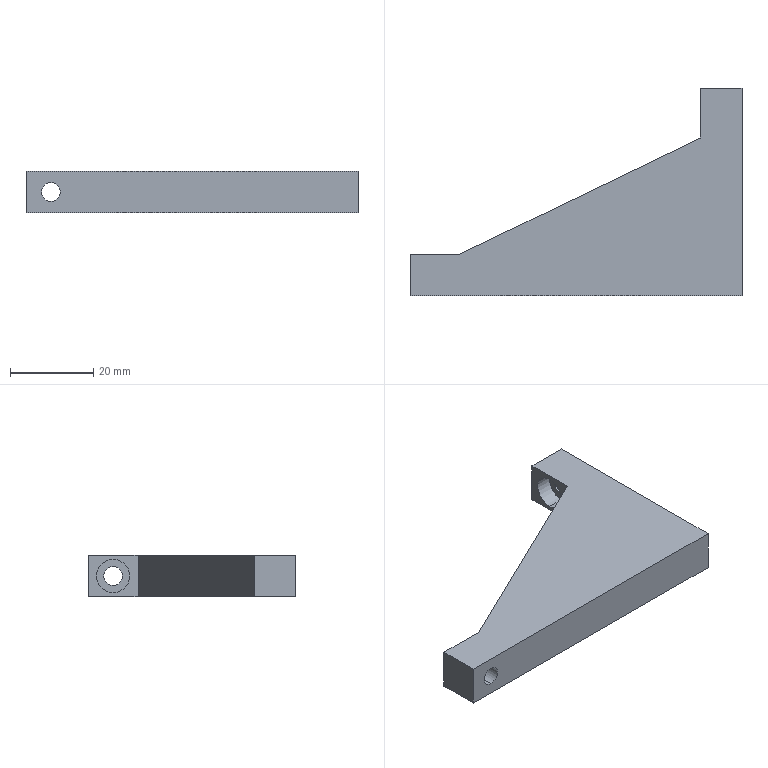Part | NX | features BREP 1 | 1 solid | 19 faces | box 80 x 50 x 10 mm | volume 19527 mm3 | plane 11 | cylinder 8 | commonest cylinder face diameters 4.5 x4 8 x4
STEP:
#1=CARTESIAN_POINT('',(-707.789,88.721,1.));
#2=VERTEX_POINT('',#1);
#3=CARTESIAN_POINT('',(-707.789,88.721,9.));
#4=VERTEX_POINT('',#3);
#5=CARTESIAN_POINT('',(-707.789,88.721,5.));
#6=DIRECTION('',(0.,1.,0.));
#7=DIRECTION('',(0.,0.,1.));
#8=AXIS2_PLACEMENT_3D('',#5,#6,#7);
#9=CIRCLE('',#8,4.);
#10=EDGE_CURVE('',#2,#4,#9,.T.);
#11=ORIENTED_EDGE('',*,*,#10,.F.);
#12=CARTESIAN_POINT('',(-707.789,92.721,1.));
#13=VERTEX_POINT('',#12);
#14=CARTESIAN_POINT('',(-707.789,92.721,1.));
#15=DIRECTION('',(0.,1.,0.));
#16=VECTOR('',#15,1000.);
#17=LINE('',#14,#16);
#18=EDGE_CURVE('',#13,#2,#17,.F.);
#19=ORIENTED_EDGE('',*,*,#18,.F.);
#20=CARTESIAN_POINT('',(-707.789,92.721,9.));
#21=VERTEX_POINT('',#20);
#22=CARTESIAN_POINT('',(-707.789,92.721,5.));
#23=DIRECTION('',(0.,1.,0.));
#24=DIRECTION('',(0.,0.,1.));
#25=AXIS2_PLACEMENT_3D('',#22,#23,#24);
#26=CIRCLE('',#25,4.);
#27=EDGE_CURVE('',#13,#21,#26,.T.);
#28=ORIENTED_EDGE('',*,*,#27,.T.);
#29=CARTESIAN_POINT('',(-707.789,92.721,9.));
#30=DIRECTION('',(0.,1.,0.));
#31=VECTOR('',#30,1000.);
#32=LINE('',#29,#31);
#33=EDGE_CURVE('',#21,#4,#32,.F.);
#34=ORIENTED_EDGE('',*,*,#33,.T.);
#35=EDGE_LOOP('',(#11,#19,#28,#34));
#36=FACE_BOUND('',#35,.T.);
#37=CARTESIAN_POINT('',(-707.789,92.721,5.));
#38=DIRECTION('',(0.,1.,0.));
#39=DIRECTION('',(0.,0.,1.));
#40=AXIS2_PLACEMENT_3D('',#37,#38,#39);
#41=CYLINDRICAL_SURFACE('',#40,4.);
#42=ADVANCED_FACE('',(#36),#41,.F.);
#43=CARTESIAN_POINT('',(-707.789,82.721,2.75));
#44=VERTEX_POINT('',#43);
#45=CARTESIAN_POINT('',(-707.789,82.721,7.25));
#46=VERTEX_POINT('',#45);
#47=CARTESIAN_POINT('',(-707.789,82.721,5.));
#48=DIRECTION('',(0.,1.,0.));
#49=DIRECTION('',(0.,0.,1.));
#50=AXIS2_PLACEMENT_3D('',#47,#48,#49);
#51=CIRCLE('',#50,2.25);
#52=EDGE_CURVE('',#44,#46,#51,.T.);
#53=ORIENTED_EDGE('',*,*,#52,.F.);
#54=CARTESIAN_POINT('',(-707.789,88.721,2.75));
#55=VERTEX_POINT('',#54);
#56=CARTESIAN_POINT('',(-707.789,92.721,2.75));
#57=DIRECTION('',(0.,1.,0.));
#58=VECTOR('',#57,1000.);
#59=LINE('',#56,#58);
#60=EDGE_CURVE('',#55,#44,#59,.F.);
#61=ORIENTED_EDGE('',*,*,#60,.F.);
#62=CARTESIAN_POINT('',(-707.789,88.721,7.25));
#63=VERTEX_POINT('',#62);
#64=CARTESIAN_POINT('',(-707.789,88.721,5.));
#65=DIRECTION('',(0.,1.,0.));
#66=DIRECTION('',(0.,0.,1.));
#67=AXIS2_PLACEMENT_3D('',#64,#65,#66);
#68=CIRCLE('',#67,2.25);
#69=EDGE_CURVE('',#55,#63,#68,.T.);
#70=ORIENTED_EDGE('',*,*,#69,.T.);
#71=CARTESIAN_POINT('',(-707.789,92.721,7.25));
#72=DIRECTION('',(0.,1.,0.));
#73=VECTOR('',#72,1000.);
#74=LINE('',#71,#73);
#75=EDGE_CURVE('',#63,#46,#74,.F.);
#76=ORIENTED_EDGE('',*,*,#75,.T.);
#77=EDGE_LOOP('',(#53,#61,#70,#76));
#78=FACE_BOUND('',#77,.T.);
#79=CARTESIAN_POINT('',(-707.789,92.721,5.));
#80=DIRECTION('',(0.,1.,0.));
#81=DIRECTION('',(0.,0.,1.));
#82=AXIS2_PLACEMENT_3D('',#79,#80,#81);
#83=CYLINDRICAL_SURFACE('',#82,2.25);
#84=ADVANCED_FACE('',(#78),#83,.F.);
#85=CARTESIAN_POINT('',(-639.789,126.721,1.));
#86=VERTEX_POINT('',#85);
#87=CARTESIAN_POINT('',(-639.789,126.721,9.));
#88=VERTEX_POINT('',#87);
#89=CARTESIAN_POINT('',(-639.789,126.721,5.));
#90=DIRECTION('',(-1.,0.,0.));
#91=DIRECTION('',(0.,0.,1.));
#92=AXIS2_PLACEMENT_3D('',#89,#90,#91);
#93=CIRCLE('',#92,4.);
#94=EDGE_CURVE('',#86,#88,#93,.T.);
#95=ORIENTED_EDGE('',*,*,#94,.F.);
#96=CARTESIAN_POINT('',(-643.789,126.721,1.));
#97=VERTEX_POINT('',#96);
#98=CARTESIAN_POINT('',(-643.789,126.721,1.));
#99=DIRECTION('',(-1.,0.,0.));
#100=VECTOR('',#99,1000.);
#101=LINE('',#98,#100);
#102=EDGE_CURVE('',#97,#86,#101,.F.);
#103=ORIENTED_EDGE('',*,*,#102,.F.);
#104=CARTESIAN_POINT('',(-643.789,126.721,9.));
#105=VERTEX_POINT('',#104);
#106=CARTESIAN_POINT('',(-643.789,126.721,5.));
#107=DIRECTION('',(-1.,0.,0.));
#108=DIRECTION('',(0.,0.,1.));
#109=AXIS2_PLACEMENT_3D('',#106,#107,#108);
#110=CIRCLE('',#109,4.);
#111=EDGE_CURVE('',#97,#105,#110,.T.);
#112=ORIENTED_EDGE('',*,*,#111,.T.);
#113=CARTESIAN_POINT('',(-643.789,126.721,9.));
#114=DIRECTION('',(-1.,0.,0.));
#115=VECTOR('',#114,1000.);
#116=LINE('',#113,#115);
#117=EDGE_CURVE('',#105,#88,#116,.F.);
#118=ORIENTED_EDGE('',*,*,#117,.T.);
#119=EDGE_LOOP('',(#95,#103,#112,#118));
#120=FACE_BOUND('',#119,.T.);
#121=CARTESIAN_POINT('',(-643.789,126.721,5.));
#122=DIRECTION('',(-1.,0.,0.));
#123=DIRECTION('',(0.,0.,1.));
#124=AXIS2_PLACEMENT_3D('',#121,#122,#123);
#125=CYLINDRICAL_SURFACE('',#124,4.);
#126=ADVANCED_FACE('',(#120),#125,.F.);
#127=CARTESIAN_POINT('',(-633.789,126.721,2.75));
#128=VERTEX_POINT('',#127);
#129=CARTESIAN_POINT('',(-633.789,126.721,7.25));
#130=VERTEX_POINT('',#129);
#131=CARTESIAN_POINT('',(-633.789,126.721,5.));
#132=DIRECTION('',(-1.,0.,0.));
#133=DIRECTION('',(0.,0.,1.));
#134=AXIS2_PLACEMENT_3D('',#131,#132,#133);
#135=CIRCLE('',#134,2.25);
#136=EDGE_CURVE('',#128,#130,#135,.T.);
#137=ORIENTED_EDGE('',*,*,#136,.F.);
#138=CARTESIAN_POINT('',(-639.789,126.721,2.75));
#139=VERTEX_POINT('',#138);
#140=CARTESIAN_POINT('',(-643.789,126.721,2.75));
#141=DIRECTION('',(-1.,0.,0.));
#142=VECTOR('',#141,1000.);
#143=LINE('',#140,#142);
#144=EDGE_CURVE('',#139,#128,#143,.F.);
#145=ORIENTED_EDGE('',*,*,#144,.F.);
#146=CARTESIAN_POINT('',(-639.789,126.721,7.25));
#147=VERTEX_POINT('',#146);
#148=CARTESIAN_POINT('',(-639.789,126.721,5.));
#149=DIRECTION('',(-1.,0.,0.));
#150=DIRECTION('',(0.,0.,1.));
#151=AXIS2_PLACEMENT_3D('',#148,#149,#150);
#152=CIRCLE('',#151,2.25);
#153=EDGE_CURVE('',#139,#147,#152,.T.);
#154=ORIENTED_EDGE('',*,*,#153,.T.);
#155=CARTESIAN_POINT('',(-643.789,126.721,7.25));
#156=DIRECTION('',(-1.,0.,0.));
#157=VECTOR('',#156,1000.);
#158=LINE('',#155,#157);
#159=EDGE_CURVE('',#147,#130,#158,.F.);
#160=ORIENTED_EDGE('',*,*,#159,.T.);
#161=EDGE_LOOP('',(#137,#145,#154,#160));
#162=FACE_BOUND('',#161,.T.);
#163=CARTESIAN_POINT('',(-643.789,126.721,5.));
#164=DIRECTION('',(-1.,0.,0.));
#165=DIRECTION('',(0.,0.,1.));
#166=AXIS2_PLACEMENT_3D('',#163,#164,#165);
#167=CYLINDRICAL_SURFACE('',#166,2.25);
#168=ADVANCED_FACE('',(#162),#167,.F.);
#169=CARTESIAN_POINT('',(-633.789,82.721,0.));
#170=VERTEX_POINT('',#169);
#171=CARTESIAN_POINT('',(-633.789,132.721,0.));
#172=VERTEX_POINT('',#171);
#173=CARTESIAN_POINT('',(-633.789,82.721,0.));
#174=DIRECTION('',(0.,1.,0.));
#175=VECTOR('',#174,1000.);
#176=LINE('',#173,#175);
#177=EDGE_CURVE('',#170,#172,#176,.T.);
#178=ORIENTED_EDGE('',*,*,#177,.T.);
#179=CARTESIAN_POINT('',(-633.789,132.721,10.));
#180=VERTEX_POINT('',#179);
#181=CARTESIAN_POINT('',(-633.789,132.721,10.));
#182=DIRECTION('',(0.,0.,-1.));
#183=VECTOR('',#182,1000.);
#184=LINE('',#181,#183);
#185=EDGE_CURVE('',#180,#172,#184,.T.);
#186=ORIENTED_EDGE('',*,*,#185,.F.);
#187=CARTESIAN_POINT('',(-633.789,82.721,10.));
#188=VERTEX_POINT('',#187);
#189=CARTESIAN_POINT('',(-633.789,82.721,10.));
#190=DIRECTION('',(0.,1.,0.));
#191=VECTOR('',#190,1000.);
#192=LINE('',#189,#191);
#193=EDGE_CURVE('',#188,#180,#192,.T.);
#194=ORIENTED_EDGE('',*,*,#193,.F.);
#195=CARTESIAN_POINT('',(-633.789,82.721,10.));
#196=DIRECTION('',(0.,0.,-1.));
#197=VECTOR('',#196,1000.);
#198=LINE('',#195,#197);
#199=EDGE_CURVE('',#188,#170,#198,.T.);
#200=ORIENTED_EDGE('',*,*,#199,.T.);
#201=EDGE_LOOP('',(#178,#186,#194,#200));
#202=FACE_BOUND('',#201,.T.);
#203=CARTESIAN_POINT('',(-633.789,126.721,5.));
#204=DIRECTION('',(-1.,0.,0.));
#205=DIRECTION('',(0.,0.,1.));
#206=AXIS2_PLACEMENT_3D('',#203,#204,#205);
#207=CIRCLE('',#206,2.25);
#208=EDGE_CURVE('',#130,#128,#207,.T.);
#209=ORIENTED_EDGE('',*,*,#208,.T.);
#210=ORIENTED_EDGE('',*,*,#136,.T.);
#211=EDGE_LOOP('',(#209,#210));
#212=FACE_BOUND('',#211,.T.);
#213=CARTESIAN_POINT('',(-633.789,82.721,10.));
#214=DIRECTION('',(-1.,0.,0.));
#215=DIRECTION('',(0.,0.,1.));
#216=AXIS2_PLACEMENT_3D('',#213,#214,#215);
#217=PLANE('',#216);
#218=ADVANCED_FACE('',(#202,#212),#217,.F.);
#219=CARTESIAN_POINT('',(-643.789,132.721,0.));
#220=VERTEX_POINT('',#219);
#221=CARTESIAN_POINT('',(-633.789,132.721,0.));
#222=DIRECTION('',(-1.,0.,0.));
#223=VECTOR('',#222,1000.);
#224=LINE('',#221,#223);
#225=EDGE_CURVE('',#172,#220,#224,.T.);
#226=ORIENTED_EDGE('',*,*,#225,.T.);
#227=CARTESIAN_POINT('',(-643.789,132.721,10.));
#228=VERTEX_POINT('',#227);
#229=CARTESIAN_POINT('',(-643.789,132.721,10.));
#230=DIRECTION('',(0.,0.,-1.));
#231=VECTOR('',#230,1000.);
#232=LINE('',#229,#231);
#233=EDGE_CURVE('',#228,#220,#232,.T.);
#234=ORIENTED_EDGE('',*,*,#233,.F.);
#235=CARTESIAN_POINT('',(-633.789,132.721,10.));
#236=DIRECTION('',(-1.,0.,0.));
#237=VECTOR('',#236,1000.);
#238=LINE('',#235,#237);
#239=EDGE_CURVE('',#180,#228,#238,.T.);
#240=ORIENTED_EDGE('',*,*,#239,.F.);
#241=ORIENTED_EDGE('',*,*,#185,.T.);
#242=EDGE_LOOP('',(#226,#234,#240,#241));
#243=FACE_BOUND('',#242,.T.);
#244=CARTESIAN_POINT('',(-633.789,132.721,10.));
#245=DIRECTION('',(0.,-1.,0.));
#246=DIRECTION('',(0.,0.,-1.));
#247=AXIS2_PLACEMENT_3D('',#244,#245,#246);
#248=PLANE('',#247);
#249=ADVANCED_FACE('',(#243),#248,.F.);
#250=CARTESIAN_POINT('',(-643.789,120.721,0.));
#251=VERTEX_POINT('',#250);
#252=CARTESIAN_POINT('',(-643.789,132.721,0.));
#253=DIRECTION('',(0.,-1.,0.));
#254=VECTOR('',#253,1000.);
#255=LINE('',#252,#254);
#256=EDGE_CURVE('',#220,#251,#255,.T.);
#257=ORIENTED_EDGE('',*,*,#256,.T.);
#258=CARTESIAN_POINT('',(-643.789,120.721,10.));
#259=VERTEX_POINT('',#258);
#260=CARTESIAN_POINT('',(-643.789,120.721,10.));
#261=DIRECTION('',(0.,0.,-1.));
#262=VECTOR('',#261,1000.);
#263=LINE('',#260,#262);
#264=EDGE_CURVE('',#259,#251,#263,.T.);
#265=ORIENTED_EDGE('',*,*,#264,.F.);
#266=CARTESIAN_POINT('',(-643.789,132.721,10.));
#267=DIRECTION('',(0.,-1.,0.));
#268=VECTOR('',#267,1000.);
#269=LINE('',#266,#268);
#270=EDGE_CURVE('',#228,#259,#269,.T.);
#271=ORIENTED_EDGE('',*,*,#270,.F.);
#272=ORIENTED_EDGE('',*,*,#233,.T.);
#273=EDGE_LOOP('',(#257,#265,#271,#272));
#274=FACE_BOUND('',#273,.T.);
#275=CARTESIAN_POINT('',(-643.789,126.721,5.));
#276=DIRECTION('',(-1.,0.,0.));
#277=DIRECTION('',(0.,0.,1.));
#278=AXIS2_PLACEMENT_3D('',#275,#276,#277);
#279=CIRCLE('',#278,4.);
#280=EDGE_CURVE('',#105,#97,#279,.T.);
#281=ORIENTED_EDGE('',*,*,#280,.F.);
#282=ORIENTED_EDGE('',*,*,#111,.F.);
#283=EDGE_LOOP('',(#281,#282));
#284=FACE_BOUND('',#283,.T.);
#285=CARTESIAN_POINT('',(-643.789,132.721,10.));
#286=DIRECTION('',(1.,0.,0.));
#287=DIRECTION('',(0.,1.,0.));
#288=AXIS2_PLACEMENT_3D('',#285,#286,#287);
#289=PLANE('',#288);
#290=ADVANCED_FACE('',(#274,#284),#289,.F.);
#291=CARTESIAN_POINT('',(-701.789,92.721,0.));
#292=VERTEX_POINT('',#291);
#293=CARTESIAN_POINT('',(-643.789,120.721,0.));
#294=DIRECTION('',(-0.9006,-0.4347,0.));
#295=VECTOR('',#294,1000.);
#296=LINE('',#293,#295);
#297=EDGE_CURVE('',#251,#292,#296,.T.);
#298=ORIENTED_EDGE('',*,*,#297,.T.);
#299=CARTESIAN_POINT('',(-701.789,92.721,10.));
#300=VERTEX_POINT('',#299);
#301=CARTESIAN_POINT('',(-701.789,92.721,10.));
#302=DIRECTION('',(0.,0.,-1.));
#303=VECTOR('',#302,1000.);
#304=LINE('',#301,#303);
#305=EDGE_CURVE('',#300,#292,#304,.T.);
#306=ORIENTED_EDGE('',*,*,#305,.F.);
#307=CARTESIAN_POINT('',(-643.789,120.721,10.));
#308=DIRECTION('',(-0.9006,-0.4347,0.));
#309=VECTOR('',#308,1000.);
#310=LINE('',#307,#309);
#311=EDGE_CURVE('',#259,#300,#310,.T.);
#312=ORIENTED_EDGE('',*,*,#311,.F.);
#313=ORIENTED_EDGE('',*,*,#264,.T.);
#314=EDGE_LOOP('',(#298,#306,#312,#313));
#315=FACE_BOUND('',#314,.T.);
#316=CARTESIAN_POINT('',(-643.789,120.721,10.));
#317=DIRECTION('',(0.4347,-0.9006,0.));
#318=DIRECTION('',(0.,0.,-1.));
#319=AXIS2_PLACEMENT_3D('',#316,#317,#318);
#320=PLANE('',#319);
#321=ADVANCED_FACE('',(#315),#320,.F.);
#322=CARTESIAN_POINT('',(-713.789,92.721,0.));
#323=VERTEX_POINT('',#322);
#324=CARTESIAN_POINT('',(-701.789,92.721,0.));
#325=DIRECTION('',(-1.,0.,0.));
#326=VECTOR('',#325,1000.);
#327=LINE('',#324,#326);
#328=EDGE_CURVE('',#292,#323,#327,.T.);
#329=ORIENTED_EDGE('',*,*,#328,.T.);
#330=CARTESIAN_POINT('',(-713.789,92.721,10.));
#331=VERTEX_POINT('',#330);
#332=CARTESIAN_POINT('',(-713.789,92.721,10.));
#333=DIRECTION('',(0.,0.,-1.));
#334=VECTOR('',#333,1000.);
#335=LINE('',#332,#334);
#336=EDGE_CURVE('',#331,#323,#335,.T.);
#337=ORIENTED_EDGE('',*,*,#336,.F.);
#338=CARTESIAN_POINT('',(-701.789,92.721,10.));
#339=DIRECTION('',(-1.,0.,0.));
#340=VECTOR('',#339,1000.);
#341=LINE('',#338,#340);
#342=EDGE_CURVE('',#300,#331,#341,.T.);
#343=ORIENTED_EDGE('',*,*,#342,.F.);
#344=ORIENTED_EDGE('',*,*,#305,.T.);
#345=EDGE_LOOP('',(#329,#337,#343,#344));
#346=FACE_BOUND('',#345,.T.);
#347=CARTESIAN_POINT('',(-707.789,92.721,5.));
#348=DIRECTION('',(0.,1.,0.));
#349=DIRECTION('',(0.,0.,1.));
#350=AXIS2_PLACEMENT_3D('',#347,#348,#349);
#351=CIRCLE('',#350,4.);
#352=EDGE_CURVE('',#21,#13,#351,.T.);
#353=ORIENTED_EDGE('',*,*,#352,.F.);
#354=ORIENTED_EDGE('',*,*,#27,.F.);
#355=EDGE_LOOP('',(#353,#354));
#356=FACE_BOUND('',#355,.T.);
#357=CARTESIAN_POINT('',(-701.789,92.721,10.));
#358=DIRECTION('',(0.,-1.,0.));
#359=DIRECTION('',(0.,0.,-1.));
#360=AXIS2_PLACEMENT_3D('',#357,#358,#359);
#361=PLANE('',#360);
#362=ADVANCED_FACE('',(#346,#356),#361,.F.);
#363=CARTESIAN_POINT('',(-713.789,82.721,0.));
#364=VERTEX_POINT('',#363);
#365=CARTESIAN_POINT('',(-713.789,92.721,0.));
#366=DIRECTION('',(0.,-1.,0.));
#367=VECTOR('',#366,1000.);
#368=LINE('',#365,#367);
#369=EDGE_CURVE('',#323,#364,#368,.T.);
#370=ORIENTED_EDGE('',*,*,#369,.T.);
#371=CARTESIAN_POINT('',(-713.789,82.721,10.));
#372=VERTEX_POINT('',#371);
#373=CARTESIAN_POINT('',(-713.789,82.721,10.));
#374=DIRECTION('',(0.,0.,-1.));
#375=VECTOR('',#374,1000.);
#376=LINE('',#373,#375);
#377=EDGE_CURVE('',#372,#364,#376,.T.);
#378=ORIENTED_EDGE('',*,*,#377,.F.);
#379=CARTESIAN_POINT('',(-713.789,92.721,10.));
#380=DIRECTION('',(0.,-1.,0.));
#381=VECTOR('',#380,1000.);
#382=LINE('',#379,#381);
#383=EDGE_CURVE('',#331,#372,#382,.T.);
#384=ORIENTED_EDGE('',*,*,#383,.F.);
#385=ORIENTED_EDGE('',*,*,#336,.T.);
#386=EDGE_LOOP('',(#370,#378,#384,#385));
#387=FACE_BOUND('',#386,.T.);
#388=CARTESIAN_POINT('',(-713.789,92.721,10.));
#389=DIRECTION('',(1.,0.,0.));
#390=DIRECTION('',(0.,1.,0.));
#391=AXIS2_PLACEMENT_3D('',#388,#389,#390);
#392=PLANE('',#391);
#393=ADVANCED_FACE('',(#387),#392,.F.);
#394=CARTESIAN_POINT('',(-713.789,82.721,0.));
#395=DIRECTION('',(1.,0.,0.));
#396=VECTOR('',#395,1000.);
#397=LINE('',#394,#396);
#398=EDGE_CURVE('',#364,#170,#397,.T.);
#399=ORIENTED_EDGE('',*,*,#398,.T.);
#400=ORIENTED_EDGE('',*,*,#199,.F.);
#401=CARTESIAN_POINT('',(-713.789,82.721,10.));
#402=DIRECTION('',(1.,0.,0.));
#403=VECTOR('',#402,1000.);
#404=LINE('',#401,#403);
#405=EDGE_CURVE('',#372,#188,#404,.T.);
#406=ORIENTED_EDGE('',*,*,#405,.F.);
#407=ORIENTED_EDGE('',*,*,#377,.T.);
#408=EDGE_LOOP('',(#399,#400,#406,#407));
#409=FACE_BOUND('',#408,.T.);
#410=CARTESIAN_POINT('',(-707.789,82.721,5.));
#411=DIRECTION('',(0.,1.,0.));
#412=DIRECTION('',(0.,0.,1.));
#413=AXIS2_PLACEMENT_3D('',#410,#411,#412);
#414=CIRCLE('',#413,2.25);
#415=EDGE_CURVE('',#46,#44,#414,.T.);
#416=ORIENTED_EDGE('',*,*,#415,.T.);
#417=ORIENTED_EDGE('',*,*,#52,.T.);
#418=EDGE_LOOP('',(#416,#417));
#419=FACE_BOUND('',#418,.T.);
#420=CARTESIAN_POINT('',(-713.789,82.721,10.));
#421=DIRECTION('',(0.,1.,0.));
#422=DIRECTION('',(1.,0.,0.));
#423=AXIS2_PLACEMENT_3D('',#420,#421,#422);
#424=PLANE('',#423);
#425=ADVANCED_FACE('',(#409,#419),#424,.F.);
#426=ORIENTED_EDGE('',*,*,#193,.T.);
#427=ORIENTED_EDGE('',*,*,#239,.T.);
#428=ORIENTED_EDGE('',*,*,#270,.T.);
#429=ORIENTED_EDGE('',*,*,#311,.T.);
#430=ORIENTED_EDGE('',*,*,#342,.T.);
#431=ORIENTED_EDGE('',*,*,#383,.T.);
#432=ORIENTED_EDGE('',*,*,#405,.T.);
#433=EDGE_LOOP('',(#426,#427,#428,#429,#430,#431,#432));
#434=FACE_BOUND('',#433,.T.);
#435=CARTESIAN_POINT('',(-633.789,132.721,10.));
#436=DIRECTION('',(0.,0.,1.));
#437=DIRECTION('',(1.,0.,0.));
#438=AXIS2_PLACEMENT_3D('',#435,#436,#437);
#439=PLANE('',#438);
#440=ADVANCED_FACE('',(#434),#439,.T.);
#441=ORIENTED_EDGE('',*,*,#177,.F.);
#442=ORIENTED_EDGE('',*,*,#398,.F.);
#443=ORIENTED_EDGE('',*,*,#369,.F.);
#444=ORIENTED_EDGE('',*,*,#328,.F.);
#445=ORIENTED_EDGE('',*,*,#297,.F.);
#446=ORIENTED_EDGE('',*,*,#256,.F.);
#447=ORIENTED_EDGE('',*,*,#225,.F.);
#448=EDGE_LOOP('',(#441,#442,#443,#444,#445,#446,#447));
#449=FACE_BOUND('',#448,.T.);
#450=CARTESIAN_POINT('',(-633.789,132.721,0.));
#451=DIRECTION('',(0.,0.,1.));
#452=DIRECTION('',(1.,0.,0.));
#453=AXIS2_PLACEMENT_3D('',#450,#451,#452);
#454=PLANE('',#453);
#455=ADVANCED_FACE('',(#449),#454,.F.);
#456=ORIENTED_EDGE('',*,*,#144,.T.);
#457=ORIENTED_EDGE('',*,*,#208,.F.);
#458=ORIENTED_EDGE('',*,*,#159,.F.);
#459=CARTESIAN_POINT('',(-639.789,126.721,5.));
#460=DIRECTION('',(-1.,0.,0.));
#461=DIRECTION('',(0.,0.,1.));
#462=AXIS2_PLACEMENT_3D('',#459,#460,#461);
#463=CIRCLE('',#462,2.25);
#464=EDGE_CURVE('',#147,#139,#463,.T.);
#465=ORIENTED_EDGE('',*,*,#464,.T.);
#466=EDGE_LOOP('',(#456,#457,#458,#465));
#467=FACE_BOUND('',#466,.T.);
#468=CARTESIAN_POINT('',(-643.789,126.721,5.));
#469=DIRECTION('',(-1.,0.,0.));
#470=DIRECTION('',(0.,0.,1.));
#471=AXIS2_PLACEMENT_3D('',#468,#469,#470);
#472=CYLINDRICAL_SURFACE('',#471,2.25);
#473=ADVANCED_FACE('',(#467),#472,.F.);
#474=CARTESIAN_POINT('',(-639.789,126.721,5.));
#475=DIRECTION('',(-1.,0.,0.));
#476=DIRECTION('',(0.,0.,1.));
#477=AXIS2_PLACEMENT_3D('',#474,#475,#476);
#478=CIRCLE('',#477,4.);
#479=EDGE_CURVE('',#88,#86,#478,.T.);
#480=ORIENTED_EDGE('',*,*,#479,.T.);
#481=ORIENTED_EDGE('',*,*,#94,.T.);
#482=EDGE_LOOP('',(#480,#481));
#483=FACE_BOUND('',#482,.T.);
#484=ORIENTED_EDGE('',*,*,#464,.F.);
#485=ORIENTED_EDGE('',*,*,#153,.F.);
#486=EDGE_LOOP('',(#484,#485));
#487=FACE_BOUND('',#486,.T.);
#488=CARTESIAN_POINT('',(-639.789,128.971,5.));
#489=DIRECTION('',(1.,0.,0.));
#490=DIRECTION('',(0.,1.,0.));
#491=AXIS2_PLACEMENT_3D('',#488,#489,#490);
#492=PLANE('',#491);
#493=ADVANCED_FACE('',(#483,#487),#492,.F.);
#494=ORIENTED_EDGE('',*,*,#102,.T.);
#495=ORIENTED_EDGE('',*,*,#479,.F.);
#496=ORIENTED_EDGE('',*,*,#117,.F.);
#497=ORIENTED_EDGE('',*,*,#280,.T.);
#498=EDGE_LOOP('',(#494,#495,#496,#497));
#499=FACE_BOUND('',#498,.T.);
#500=CARTESIAN_POINT('',(-643.789,126.721,5.));
#501=DIRECTION('',(-1.,0.,0.));
#502=DIRECTION('',(0.,0.,1.));
#503=AXIS2_PLACEMENT_3D('',#500,#501,#502);
#504=CYLINDRICAL_SURFACE('',#503,4.);
#505=ADVANCED_FACE('',(#499),#504,.F.);
#506=ORIENTED_EDGE('',*,*,#60,.T.);
#507=ORIENTED_EDGE('',*,*,#415,.F.);
#508=ORIENTED_EDGE('',*,*,#75,.F.);
#509=CARTESIAN_POINT('',(-707.789,88.721,5.));
#510=DIRECTION('',(0.,1.,0.));
#511=DIRECTION('',(0.,0.,1.));
#512=AXIS2_PLACEMENT_3D('',#509,#510,#511);
#513=CIRCLE('',#512,2.25);
#514=EDGE_CURVE('',#63,#55,#513,.T.);
#515=ORIENTED_EDGE('',*,*,#514,.T.);
#516=EDGE_LOOP('',(#506,#507,#508,#515));
#517=FACE_BOUND('',#516,.T.);
#518=CARTESIAN_POINT('',(-707.789,92.721,5.));
#519=DIRECTION('',(0.,1.,0.));
#520=DIRECTION('',(0.,0.,1.));
#521=AXIS2_PLACEMENT_3D('',#518,#519,#520);
#522=CYLINDRICAL_SURFACE('',#521,2.25);
#523=ADVANCED_FACE('',(#517),#522,.F.);
#524=CARTESIAN_POINT('',(-707.789,88.721,5.));
#525=DIRECTION('',(0.,1.,0.));
#526=DIRECTION('',(0.,0.,1.));
#527=AXIS2_PLACEMENT_3D('',#524,#525,#526);
#528=CIRCLE('',#527,4.);
#529=EDGE_CURVE('',#4,#2,#528,.T.);
#530=ORIENTED_EDGE('',*,*,#529,.T.);
#531=ORIENTED_EDGE('',*,*,#10,.T.);
#532=EDGE_LOOP('',(#530,#531));
#533=FACE_BOUND('',#532,.T.);
#534=ORIENTED_EDGE('',*,*,#514,.F.);
#535=ORIENTED_EDGE('',*,*,#69,.F.);
#536=EDGE_LOOP('',(#534,#535));
#537=FACE_BOUND('',#536,.T.);
#538=CARTESIAN_POINT('',(-705.539,88.721,5.));
#539=DIRECTION('',(0.,-1.,0.));
#540=DIRECTION('',(0.,0.,-1.));
#541=AXIS2_PLACEMENT_3D('',#538,#539,#540);
#542=PLANE('',#541);
#543=ADVANCED_FACE('',(#533,#537),#542,.F.);
#544=ORIENTED_EDGE('',*,*,#18,.T.);
#545=ORIENTED_EDGE('',*,*,#529,.F.);
#546=ORIENTED_EDGE('',*,*,#33,.F.);
#547=ORIENTED_EDGE('',*,*,#352,.T.);
#548=EDGE_LOOP('',(#544,#545,#546,#547));
#549=FACE_BOUND('',#548,.T.);
#550=CARTESIAN_POINT('',(-707.789,92.721,5.));
#551=DIRECTION('',(0.,1.,0.));
#552=DIRECTION('',(0.,0.,1.));
#553=AXIS2_PLACEMENT_3D('',#550,#551,#552);
#554=CYLINDRICAL_SURFACE('',#553,4.);
#555=ADVANCED_FACE('',(#549),#554,.F.);
#556=CLOSED_SHELL('',(#42,#84,#126,#168,#218,#249,#290,#321,#362,#393,#425,#440,#455,#473,#493,#505,#523,#543,#555));
#557=MANIFOLD_SOLID_BREP('',#556);
#558=(LENGTH_UNIT()NAMED_UNIT(*)SI_UNIT(.MILLI.,.METRE.));
#559=UNCERTAINTY_MEASURE_WITH_UNIT(LENGTH_MEASURE(0.00001),#558,'','');
#560=(NAMED_UNIT(*)PLANE_ANGLE_UNIT()SI_UNIT($,.RADIAN.));
#561=(NAMED_UNIT(*)SI_UNIT($,.STERADIAN.)SOLID_ANGLE_UNIT());
#562=(GEOMETRIC_REPRESENTATION_CONTEXT(3)GLOBAL_UNCERTAINTY_ASSIGNED_CONTEXT((#559))GLOBAL_UNIT_ASSIGNED_CONTEXT((#558,#560,#561))REPRESENTATION_CONTEXT('',''));
#563=ADVANCED_BREP_SHAPE_REPRESENTATION('',(#557),#562);